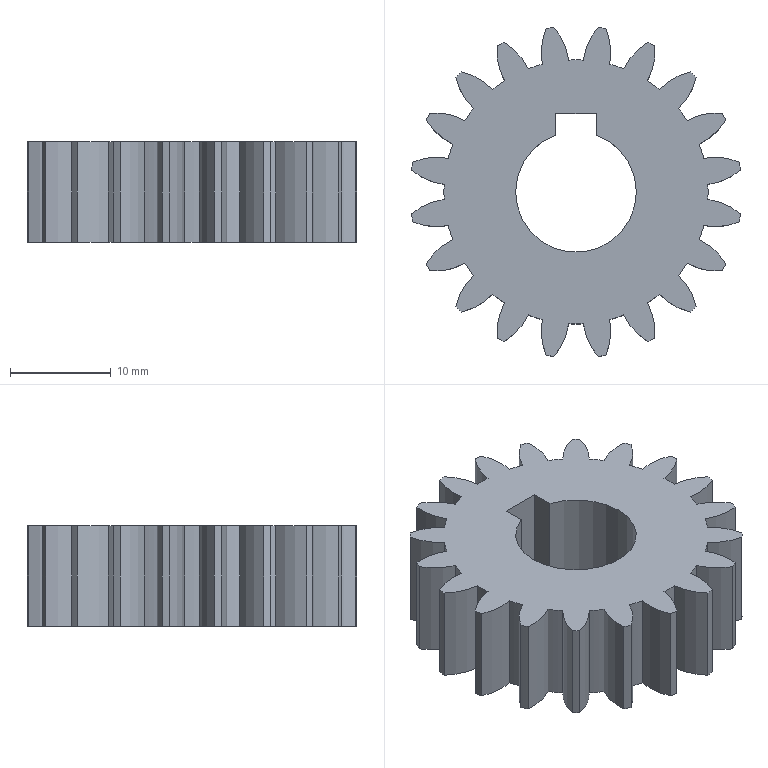Part | NX | features BREP 1 | 1 solid | 86 faces | box 32.708 x 32.708 x 10 mm | volume 5614 mm3 | cylinder 81 | plane 5 | commonest cylinder face diameters 12 x41 26.248 x20 33 x20